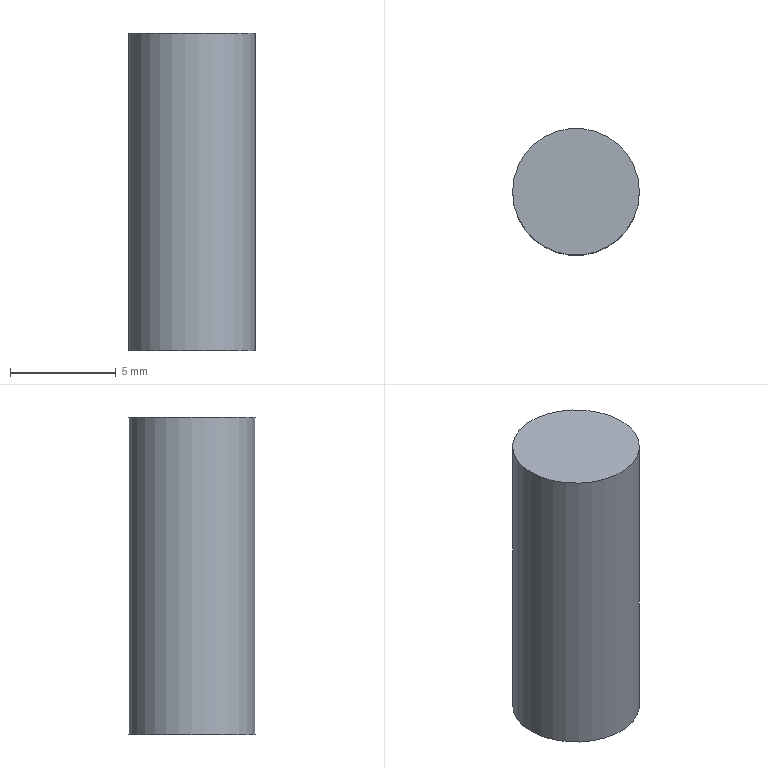Part | NX | features BREP 1 | 1 solid | 3 faces | box 6 x 6 x 15 mm | volume 424.115 mm3 | plane 2 | cylinder 1 | commonest cylinder face diameters 6 x1
STEP:
#1=CARTESIAN_POINT('',(3.,0.,-40.6));
#2=VERTEX_POINT('',#1);
#3=CARTESIAN_POINT('',(0.,0.,-40.6));
#4=DIRECTION('',(0.,0.,-1.));
#5=DIRECTION('',(1.,0.,0.));
#6=AXIS2_PLACEMENT_3D('',#3,#4,#5);
#7=CIRCLE('',#6,3.);
#8=EDGE_CURVE('',#2,#2,#7,.T.);
#9=ORIENTED_EDGE('',*,*,#8,.F.);
#10=EDGE_LOOP('',(#9));
#11=FACE_BOUND('',#10,.T.);
#12=CARTESIAN_POINT('',(3.,0.,-25.6));
#13=VERTEX_POINT('',#12);
#14=CARTESIAN_POINT('',(0.,0.,-25.6));
#15=DIRECTION('',(0.,0.,-1.));
#16=DIRECTION('',(1.,0.,0.));
#17=AXIS2_PLACEMENT_3D('',#14,#15,#16);
#18=CIRCLE('',#17,3.);
#19=EDGE_CURVE('',#13,#13,#18,.T.);
#20=ORIENTED_EDGE('',*,*,#19,.T.);
#21=EDGE_LOOP('',(#20));
#22=FACE_BOUND('',#21,.T.);
#23=CARTESIAN_POINT('',(0.,0.,-40.6));
#24=DIRECTION('',(0.,0.,1.));
#25=DIRECTION('',(-1.,0.,0.));
#26=AXIS2_PLACEMENT_3D('',#23,#24,#25);
#27=CYLINDRICAL_SURFACE('',#26,3.);
#28=ADVANCED_FACE('',(#11,#22),#27,.T.);
#29=ORIENTED_EDGE('',*,*,#8,.T.);
#30=EDGE_LOOP('',(#29));
#31=FACE_BOUND('',#30,.T.);
#32=CARTESIAN_POINT('',(0.,0.,-40.6));
#33=DIRECTION('',(0.,0.,-1.));
#34=DIRECTION('',(1.,0.,0.));
#35=AXIS2_PLACEMENT_3D('',#32,#33,#34);
#36=PLANE('',#35);
#37=ADVANCED_FACE('',(#31),#36,.T.);
#38=ORIENTED_EDGE('',*,*,#19,.F.);
#39=EDGE_LOOP('',(#38));
#40=FACE_BOUND('',#39,.T.);
#41=CARTESIAN_POINT('',(0.,0.,-25.6));
#42=DIRECTION('',(0.,0.,-1.));
#43=DIRECTION('',(1.,0.,0.));
#44=AXIS2_PLACEMENT_3D('',#41,#42,#43);
#45=PLANE('',#44);
#46=ADVANCED_FACE('',(#40),#45,.F.);
#47=CLOSED_SHELL('',(#28,#37,#46));
#48=MANIFOLD_SOLID_BREP('',#47);
#49=(LENGTH_UNIT()NAMED_UNIT(*)SI_UNIT(.MILLI.,.METRE.));
#50=UNCERTAINTY_MEASURE_WITH_UNIT(LENGTH_MEASURE(0.00001),#49,'','');
#51=(NAMED_UNIT(*)PLANE_ANGLE_UNIT()SI_UNIT($,.RADIAN.));
#52=(NAMED_UNIT(*)SI_UNIT($,.STERADIAN.)SOLID_ANGLE_UNIT());
#53=(GEOMETRIC_REPRESENTATION_CONTEXT(3)GLOBAL_UNCERTAINTY_ASSIGNED_CONTEXT((#50))GLOBAL_UNIT_ASSIGNED_CONTEXT((#49,#51,#52))REPRESENTATION_CONTEXT('',''));
#54=ADVANCED_BREP_SHAPE_REPRESENTATION('',(#48),#53);